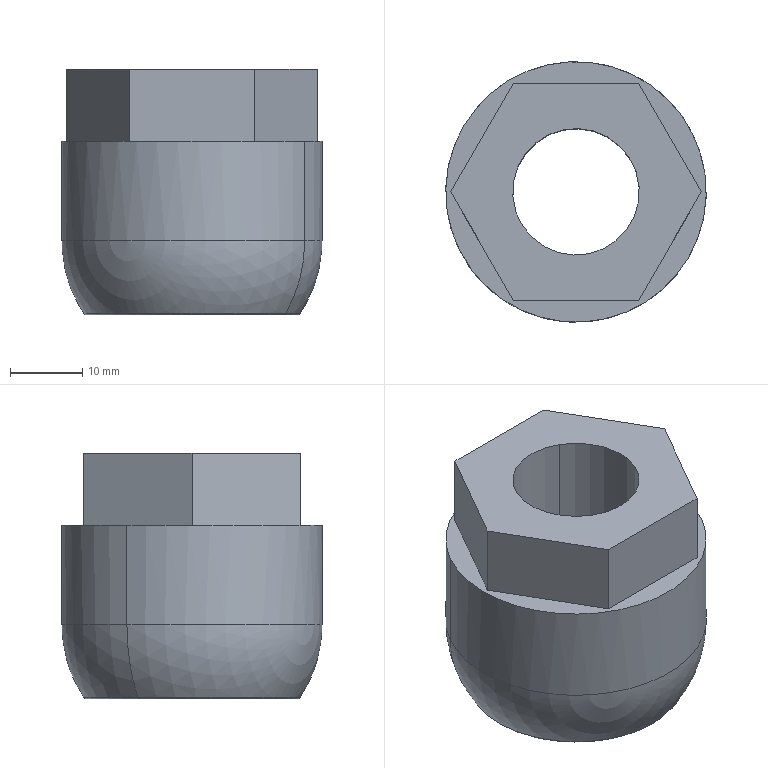Part | NX | 1 solid | 17 faces | box 36 x 36 x 34 mm | volume 22917 mm3 | plane 9 | cylinder 4 | torus 2 | sphere 2 | commonest cylinder face diameters 17.5 x2 36 x2
STEP:
#1=CARTESIAN_POINT('',(-4.375,-7.578,-34.));
#2=VERTEX_POINT('',#1);
#3=CARTESIAN_POINT('',(4.375,7.578,-34.));
#4=VERTEX_POINT('',#3);
#5=CARTESIAN_POINT('',(0.,0.,-34.));
#6=DIRECTION('',(0.,0.,1.));
#7=DIRECTION('',(0.5,0.866,0.));
#8=AXIS2_PLACEMENT_3D('',#5,#6,#7);
#9=CIRCLE('',#8,8.75);
#10=EDGE_CURVE('',#2,#4,#9,.T.);
#11=ORIENTED_EDGE('',*,*,#10,.F.);
#12=CARTESIAN_POINT('',(-4.375,-7.578,0.));
#13=VERTEX_POINT('',#12);
#14=CARTESIAN_POINT('',(-4.375,-7.578,0.));
#15=DIRECTION('',(0.,0.,1.));
#16=VECTOR('',#15,1000.);
#17=LINE('',#14,#16);
#18=EDGE_CURVE('',#13,#2,#17,.F.);
#19=ORIENTED_EDGE('',*,*,#18,.F.);
#20=CARTESIAN_POINT('',(4.375,7.578,0.));
#21=VERTEX_POINT('',#20);
#22=CARTESIAN_POINT('',(0.,0.,0.));
#23=DIRECTION('',(0.,0.,1.));
#24=DIRECTION('',(0.5,0.866,0.));
#25=AXIS2_PLACEMENT_3D('',#22,#23,#24);
#26=CIRCLE('',#25,8.75);
#27=EDGE_CURVE('',#13,#21,#26,.T.);
#28=ORIENTED_EDGE('',*,*,#27,.T.);
#29=CARTESIAN_POINT('',(4.375,7.578,0.));
#30=DIRECTION('',(0.,0.,1.));
#31=VECTOR('',#30,1000.);
#32=LINE('',#29,#31);
#33=EDGE_CURVE('',#21,#4,#32,.F.);
#34=ORIENTED_EDGE('',*,*,#33,.T.);
#35=EDGE_LOOP('',(#11,#19,#28,#34));
#36=FACE_BOUND('',#35,.T.);
#37=CARTESIAN_POINT('',(0.,0.,0.));
#38=DIRECTION('',(0.,0.,1.));
#39=DIRECTION('',(-0.5,-0.866,0.));
#40=AXIS2_PLACEMENT_3D('',#37,#38,#39);
#41=CYLINDRICAL_SURFACE('',#40,8.75);
#42=ADVANCED_FACE('',(#36),#41,.F.);
#43=CARTESIAN_POINT('',(-12.586,7.267,-34.));
#44=VERTEX_POINT('',#43);
#45=CARTESIAN_POINT('',(12.586,-7.267,-34.));
#46=VERTEX_POINT('',#45);
#47=CARTESIAN_POINT('',(0.,0.,-34.));
#48=DIRECTION('',(0.,0.,1.));
#49=DIRECTION('',(-0.866,0.5,0.));
#50=AXIS2_PLACEMENT_3D('',#47,#48,#49);
#51=CIRCLE('',#50,14.533);
#52=EDGE_CURVE('',#44,#46,#51,.T.);
#53=ORIENTED_EDGE('',*,*,#52,.T.);
#54=CARTESIAN_POINT('',(12.946,-7.474,-33.779));
#55=VERTEX_POINT('',#54);
#56=CARTESIAN_POINT('',(12.586,-7.267,-33.5));
#57=DIRECTION('',(-0.5,-0.866,0.));
#58=DIRECTION('',(-0.866,0.5,0.));
#59=AXIS2_PLACEMENT_3D('',#56,#57,#58);
#60=CIRCLE('',#59,0.5);
#61=EDGE_CURVE('',#55,#46,#60,.F.);
#62=ORIENTED_EDGE('',*,*,#61,.F.);
#63=CARTESIAN_POINT('',(-12.946,7.474,-33.779));
#64=VERTEX_POINT('',#63);
#65=CARTESIAN_POINT('',(0.,0.,-33.779));
#66=DIRECTION('',(0.,0.,1.));
#67=DIRECTION('',(-0.866,0.5,0.));
#68=AXIS2_PLACEMENT_3D('',#65,#66,#67);
#69=CIRCLE('',#68,14.948);
#70=EDGE_CURVE('',#64,#55,#69,.T.);
#71=ORIENTED_EDGE('',*,*,#70,.F.);
#72=CARTESIAN_POINT('',(-12.586,7.267,-33.5));
#73=DIRECTION('',(0.5,0.866,0.));
#74=DIRECTION('',(0.866,-0.5,0.));
#75=AXIS2_PLACEMENT_3D('',#72,#73,#74);
#76=CIRCLE('',#75,0.5);
#77=EDGE_CURVE('',#64,#44,#76,.F.);
#78=ORIENTED_EDGE('',*,*,#77,.T.);
#79=EDGE_LOOP('',(#53,#62,#71,#78));
#80=FACE_BOUND('',#79,.T.);
#81=CARTESIAN_POINT('',(0.,0.,-33.5));
#82=DIRECTION('',(0.,0.,1.));
#83=DIRECTION('',(0.866,-0.5,0.));
#84=AXIS2_PLACEMENT_3D('',#81,#82,#83);
#85=TOROIDAL_SURFACE('',#84,14.533,0.5);
#86=ADVANCED_FACE('',(#80),#85,.T.);
#87=ORIENTED_EDGE('',*,*,#70,.T.);
#88=CARTESIAN_POINT('',(15.588,-9.,-23.751));
#89=VERTEX_POINT('',#88);
#90=CARTESIAN_POINT('',(0.,0.,-23.751));
#91=DIRECTION('',(-0.5,-0.866,0.));
#92=DIRECTION('',(-0.866,0.5,0.));
#93=AXIS2_PLACEMENT_3D('',#90,#91,#92);
#94=CIRCLE('',#93,18.);
#95=EDGE_CURVE('',#89,#55,#94,.F.);
#96=ORIENTED_EDGE('',*,*,#95,.F.);
#97=CARTESIAN_POINT('',(-15.588,9.,-23.751));
#98=VERTEX_POINT('',#97);
#99=CARTESIAN_POINT('',(0.,0.,-23.751));
#100=DIRECTION('',(0.,0.,1.));
#101=DIRECTION('',(-0.866,0.5,0.));
#102=AXIS2_PLACEMENT_3D('',#99,#100,#101);
#103=CIRCLE('',#102,18.);
#104=EDGE_CURVE('',#98,#89,#103,.T.);
#105=ORIENTED_EDGE('',*,*,#104,.F.);
#106=CARTESIAN_POINT('',(0.,0.,-23.751));
#107=DIRECTION('',(0.5,0.866,0.));
#108=DIRECTION('',(0.866,-0.5,0.));
#109=AXIS2_PLACEMENT_3D('',#106,#107,#108);
#110=CIRCLE('',#109,18.);
#111=EDGE_CURVE('',#98,#64,#110,.F.);
#112=ORIENTED_EDGE('',*,*,#111,.T.);
#113=EDGE_LOOP('',(#87,#96,#105,#112));
#114=FACE_BOUND('',#113,.T.);
#115=CARTESIAN_POINT('',(0.,0.,-23.751));
#116=DIRECTION('',(-0.5,-0.866,0.));
#117=DIRECTION('',(0.866,-0.5,0.));
#118=AXIS2_PLACEMENT_3D('',#115,#116,#117);
#119=SPHERICAL_SURFACE('',#118,18.);
#120=ADVANCED_FACE('',(#114),#119,.T.);
#121=ORIENTED_EDGE('',*,*,#104,.T.);
#122=CARTESIAN_POINT('',(15.588,-9.,-10.));
#123=VERTEX_POINT('',#122);
#124=CARTESIAN_POINT('',(15.588,-9.,-35.614));
#125=DIRECTION('',(0.,0.,1.));
#126=VECTOR('',#125,1000.);
#127=LINE('',#124,#126);
#128=EDGE_CURVE('',#123,#89,#127,.F.);
#129=ORIENTED_EDGE('',*,*,#128,.F.);
#130=CARTESIAN_POINT('',(-15.588,9.,-10.));
#131=VERTEX_POINT('',#130);
#132=CARTESIAN_POINT('',(0.,0.,-10.));
#133=DIRECTION('',(0.,0.,-1.));
#134=DIRECTION('',(-0.866,0.5,0.));
#135=AXIS2_PLACEMENT_3D('',#132,#133,#134);
#136=CIRCLE('',#135,18.);
#137=EDGE_CURVE('',#123,#131,#136,.T.);
#138=ORIENTED_EDGE('',*,*,#137,.T.);
#139=CARTESIAN_POINT('',(-15.588,9.,-35.614));
#140=DIRECTION('',(0.,0.,1.));
#141=VECTOR('',#140,1000.);
#142=LINE('',#139,#141);
#143=EDGE_CURVE('',#131,#98,#142,.F.);
#144=ORIENTED_EDGE('',*,*,#143,.T.);
#145=EDGE_LOOP('',(#121,#129,#138,#144));
#146=FACE_BOUND('',#145,.T.);
#147=CARTESIAN_POINT('',(0.,0.,-35.614));
#148=DIRECTION('',(0.,0.,1.));
#149=DIRECTION('',(0.866,-0.5,0.));
#150=AXIS2_PLACEMENT_3D('',#147,#148,#149);
#151=CYLINDRICAL_SURFACE('',#150,18.);
#152=ADVANCED_FACE('',(#146),#151,.T.);
#153=ORIENTED_EDGE('',*,*,#128,.T.);
#154=CARTESIAN_POINT('',(0.,0.,-23.751));
#155=DIRECTION('',(0.,0.,1.));
#156=DIRECTION('',(-0.866,0.5,0.));
#157=AXIS2_PLACEMENT_3D('',#154,#155,#156);
#158=CIRCLE('',#157,18.);
#159=EDGE_CURVE('',#89,#98,#158,.T.);
#160=ORIENTED_EDGE('',*,*,#159,.T.);
#161=ORIENTED_EDGE('',*,*,#143,.F.);
#162=CARTESIAN_POINT('',(0.,0.,-10.));
#163=DIRECTION('',(0.,0.,-1.));
#164=DIRECTION('',(-0.866,0.5,0.));
#165=AXIS2_PLACEMENT_3D('',#162,#163,#164);
#166=CIRCLE('',#165,18.);
#167=EDGE_CURVE('',#131,#123,#166,.T.);
#168=ORIENTED_EDGE('',*,*,#167,.T.);
#169=EDGE_LOOP('',(#153,#160,#161,#168));
#170=FACE_BOUND('',#169,.T.);
#171=CARTESIAN_POINT('',(0.,0.,-35.614));
#172=DIRECTION('',(0.,0.,1.));
#173=DIRECTION('',(0.866,-0.5,0.));
#174=AXIS2_PLACEMENT_3D('',#171,#172,#173);
#175=CYLINDRICAL_SURFACE('',#174,18.);
#176=ADVANCED_FACE('',(#170),#175,.T.);
#177=CARTESIAN_POINT('',(0.,0.,0.));
#178=DIRECTION('',(0.,0.,1.));
#179=DIRECTION('',(0.5,0.866,0.));
#180=AXIS2_PLACEMENT_3D('',#177,#178,#179);
#181=CIRCLE('',#180,8.75);
#182=EDGE_CURVE('',#21,#13,#181,.T.);
#183=ORIENTED_EDGE('',*,*,#182,.F.);
#184=ORIENTED_EDGE('',*,*,#27,.F.);
#185=EDGE_LOOP('',(#183,#184));
#186=FACE_BOUND('',#185,.T.);
#187=CARTESIAN_POINT('',(-8.66,15.,0.));
#188=VERTEX_POINT('',#187);
#189=CARTESIAN_POINT('',(-17.32,0.,0.));
#190=VERTEX_POINT('',#189);
#191=CARTESIAN_POINT('',(-8.66,15.,0.));
#192=DIRECTION('',(-0.5,-0.866,0.));
#193=VECTOR('',#192,1000.);
#194=LINE('',#191,#193);
#195=EDGE_CURVE('',#188,#190,#194,.T.);
#196=ORIENTED_EDGE('',*,*,#195,.T.);
#197=CARTESIAN_POINT('',(-8.66,-15.,0.));
#198=VERTEX_POINT('',#197);
#199=CARTESIAN_POINT('',(-17.32,0.,0.));
#200=DIRECTION('',(0.5,-0.866,0.));
#201=VECTOR('',#200,1000.);
#202=LINE('',#199,#201);
#203=EDGE_CURVE('',#190,#198,#202,.T.);
#204=ORIENTED_EDGE('',*,*,#203,.T.);
#205=CARTESIAN_POINT('',(8.66,-15.,0.));
#206=VERTEX_POINT('',#205);
#207=CARTESIAN_POINT('',(-8.66,-15.,0.));
#208=DIRECTION('',(1.,0.,0.));
#209=VECTOR('',#208,1000.);
#210=LINE('',#207,#209);
#211=EDGE_CURVE('',#198,#206,#210,.T.);
#212=ORIENTED_EDGE('',*,*,#211,.T.);
#213=CARTESIAN_POINT('',(17.32,0.,0.));
#214=VERTEX_POINT('',#213);
#215=CARTESIAN_POINT('',(8.66,-15.,0.));
#216=DIRECTION('',(0.5,0.866,0.));
#217=VECTOR('',#216,1000.);
#218=LINE('',#215,#217);
#219=EDGE_CURVE('',#206,#214,#218,.T.);
#220=ORIENTED_EDGE('',*,*,#219,.T.);
#221=CARTESIAN_POINT('',(8.66,15.,0.));
#222=VERTEX_POINT('',#221);
#223=CARTESIAN_POINT('',(17.32,0.,0.));
#224=DIRECTION('',(-0.5,0.866,0.));
#225=VECTOR('',#224,1000.);
#226=LINE('',#223,#225);
#227=EDGE_CURVE('',#214,#222,#226,.T.);
#228=ORIENTED_EDGE('',*,*,#227,.T.);
#229=CARTESIAN_POINT('',(8.66,15.,0.));
#230=DIRECTION('',(-1.,0.,0.));
#231=VECTOR('',#230,1000.);
#232=LINE('',#229,#231);
#233=EDGE_CURVE('',#222,#188,#232,.T.);
#234=ORIENTED_EDGE('',*,*,#233,.T.);
#235=EDGE_LOOP('',(#196,#204,#212,#220,#228,#234));
#236=FACE_BOUND('',#235,.T.);
#237=CARTESIAN_POINT('',(0.,0.,0.));
#238=DIRECTION('',(0.,0.,1.));
#239=DIRECTION('',(0.866,-0.5,0.));
#240=AXIS2_PLACEMENT_3D('',#237,#238,#239);
#241=PLANE('',#240);
#242=ADVANCED_FACE('',(#186,#236),#241,.T.);
#243=ORIENTED_EDGE('',*,*,#95,.T.);
#244=CARTESIAN_POINT('',(0.,0.,-33.779));
#245=DIRECTION('',(0.,0.,1.));
#246=DIRECTION('',(-0.866,0.5,0.));
#247=AXIS2_PLACEMENT_3D('',#244,#245,#246);
#248=CIRCLE('',#247,14.948);
#249=EDGE_CURVE('',#55,#64,#248,.T.);
#250=ORIENTED_EDGE('',*,*,#249,.T.);
#251=ORIENTED_EDGE('',*,*,#111,.F.);
#252=ORIENTED_EDGE('',*,*,#159,.F.);
#253=EDGE_LOOP('',(#243,#250,#251,#252));
#254=FACE_BOUND('',#253,.T.);
#255=CARTESIAN_POINT('',(0.,0.,-23.751));
#256=DIRECTION('',(-0.5,-0.866,0.));
#257=DIRECTION('',(0.866,-0.5,0.));
#258=AXIS2_PLACEMENT_3D('',#255,#256,#257);
#259=SPHERICAL_SURFACE('',#258,18.);
#260=ADVANCED_FACE('',(#254),#259,.T.);
#261=ORIENTED_EDGE('',*,*,#61,.T.);
#262=CARTESIAN_POINT('',(0.,0.,-34.));
#263=DIRECTION('',(0.,0.,1.));
#264=DIRECTION('',(-0.866,0.5,0.));
#265=AXIS2_PLACEMENT_3D('',#262,#263,#264);
#266=CIRCLE('',#265,14.533);
#267=EDGE_CURVE('',#46,#44,#266,.T.);
#268=ORIENTED_EDGE('',*,*,#267,.T.);
#269=ORIENTED_EDGE('',*,*,#77,.F.);
#270=ORIENTED_EDGE('',*,*,#249,.F.);
#271=EDGE_LOOP('',(#261,#268,#269,#270));
#272=FACE_BOUND('',#271,.T.);
#273=CARTESIAN_POINT('',(0.,0.,-33.5));
#274=DIRECTION('',(0.,0.,1.));
#275=DIRECTION('',(0.866,-0.5,0.));
#276=AXIS2_PLACEMENT_3D('',#273,#274,#275);
#277=TOROIDAL_SURFACE('',#276,14.533,0.5);
#278=ADVANCED_FACE('',(#272),#277,.T.);
#279=CARTESIAN_POINT('',(0.,0.,-34.));
#280=DIRECTION('',(0.,0.,1.));
#281=DIRECTION('',(0.5,0.866,0.));
#282=AXIS2_PLACEMENT_3D('',#279,#280,#281);
#283=CIRCLE('',#282,8.75);
#284=EDGE_CURVE('',#4,#2,#283,.T.);
#285=ORIENTED_EDGE('',*,*,#284,.T.);
#286=ORIENTED_EDGE('',*,*,#10,.T.);
#287=EDGE_LOOP('',(#285,#286));
#288=FACE_BOUND('',#287,.T.);
#289=ORIENTED_EDGE('',*,*,#52,.F.);
#290=ORIENTED_EDGE('',*,*,#267,.F.);
#291=EDGE_LOOP('',(#289,#290));
#292=FACE_BOUND('',#291,.T.);
#293=CARTESIAN_POINT('',(-12.586,7.267,-34.));
#294=DIRECTION('',(0.,0.,-1.));
#295=DIRECTION('',(-0.866,0.5,0.));
#296=AXIS2_PLACEMENT_3D('',#293,#294,#295);
#297=PLANE('',#296);
#298=ADVANCED_FACE('',(#288,#292),#297,.T.);
#299=ORIENTED_EDGE('',*,*,#18,.T.);
#300=ORIENTED_EDGE('',*,*,#284,.F.);
#301=ORIENTED_EDGE('',*,*,#33,.F.);
#302=ORIENTED_EDGE('',*,*,#182,.T.);
#303=EDGE_LOOP('',(#299,#300,#301,#302));
#304=FACE_BOUND('',#303,.T.);
#305=CARTESIAN_POINT('',(0.,0.,0.));
#306=DIRECTION('',(0.,0.,1.));
#307=DIRECTION('',(-0.5,-0.866,0.));
#308=AXIS2_PLACEMENT_3D('',#305,#306,#307);
#309=CYLINDRICAL_SURFACE('',#308,8.75);
#310=ADVANCED_FACE('',(#304),#309,.F.);
#311=ORIENTED_EDGE('',*,*,#167,.F.);
#312=ORIENTED_EDGE('',*,*,#137,.F.);
#313=EDGE_LOOP('',(#311,#312));
#314=FACE_BOUND('',#313,.T.);
#315=CARTESIAN_POINT('',(-8.66,15.,-10.));
#316=VERTEX_POINT('',#315);
#317=CARTESIAN_POINT('',(-17.32,0.,-10.));
#318=VERTEX_POINT('',#317);
#319=CARTESIAN_POINT('',(-8.66,15.,-10.));
#320=DIRECTION('',(-0.5,-0.866,0.));
#321=VECTOR('',#320,1000.);
#322=LINE('',#319,#321);
#323=EDGE_CURVE('',#316,#318,#322,.T.);
#324=ORIENTED_EDGE('',*,*,#323,.F.);
#325=CARTESIAN_POINT('',(8.66,15.,-10.));
#326=VERTEX_POINT('',#325);
#327=CARTESIAN_POINT('',(8.66,15.,-10.));
#328=DIRECTION('',(-1.,0.,0.));
#329=VECTOR('',#328,1000.);
#330=LINE('',#327,#329);
#331=EDGE_CURVE('',#326,#316,#330,.T.);
#332=ORIENTED_EDGE('',*,*,#331,.F.);
#333=CARTESIAN_POINT('',(17.32,0.,-10.));
#334=VERTEX_POINT('',#333);
#335=CARTESIAN_POINT('',(17.32,0.,-10.));
#336=DIRECTION('',(-0.5,0.866,0.));
#337=VECTOR('',#336,1000.);
#338=LINE('',#335,#337);
#339=EDGE_CURVE('',#334,#326,#338,.T.);
#340=ORIENTED_EDGE('',*,*,#339,.F.);
#341=CARTESIAN_POINT('',(8.66,-15.,-10.));
#342=VERTEX_POINT('',#341);
#343=CARTESIAN_POINT('',(8.66,-15.,-10.));
#344=DIRECTION('',(0.5,0.866,0.));
#345=VECTOR('',#344,1000.);
#346=LINE('',#343,#345);
#347=EDGE_CURVE('',#342,#334,#346,.T.);
#348=ORIENTED_EDGE('',*,*,#347,.F.);
#349=CARTESIAN_POINT('',(-8.66,-15.,-10.));
#350=VERTEX_POINT('',#349);
#351=CARTESIAN_POINT('',(-8.66,-15.,-10.));
#352=DIRECTION('',(1.,0.,0.));
#353=VECTOR('',#352,1000.);
#354=LINE('',#351,#353);
#355=EDGE_CURVE('',#350,#342,#354,.T.);
#356=ORIENTED_EDGE('',*,*,#355,.F.);
#357=CARTESIAN_POINT('',(-17.32,0.,-10.));
#358=DIRECTION('',(0.5,-0.866,0.));
#359=VECTOR('',#358,1000.);
#360=LINE('',#357,#359);
#361=EDGE_CURVE('',#318,#350,#360,.T.);
#362=ORIENTED_EDGE('',*,*,#361,.F.);
#363=EDGE_LOOP('',(#324,#332,#340,#348,#356,#362));
#364=FACE_BOUND('',#363,.T.);
#365=CARTESIAN_POINT('',(0.,0.,-10.));
#366=DIRECTION('',(0.,0.,1.));
#367=DIRECTION('',(0.866,-0.5,0.));
#368=AXIS2_PLACEMENT_3D('',#365,#366,#367);
#369=PLANE('',#368);
#370=ADVANCED_FACE('',(#314,#364),#369,.T.);
#371=ORIENTED_EDGE('',*,*,#203,.F.);
#372=CARTESIAN_POINT('',(-17.32,0.,-10.));
#373=DIRECTION('',(0.,0.,1.));
#374=VECTOR('',#373,1000.);
#375=LINE('',#372,#374);
#376=EDGE_CURVE('',#318,#190,#375,.T.);
#377=ORIENTED_EDGE('',*,*,#376,.F.);
#378=ORIENTED_EDGE('',*,*,#361,.T.);
#379=CARTESIAN_POINT('',(-8.66,-15.,-10.));
#380=DIRECTION('',(0.,0.,1.));
#381=VECTOR('',#380,1000.);
#382=LINE('',#379,#381);
#383=EDGE_CURVE('',#350,#198,#382,.T.);
#384=ORIENTED_EDGE('',*,*,#383,.T.);
#385=EDGE_LOOP('',(#371,#377,#378,#384));
#386=FACE_BOUND('',#385,.T.);
#387=CARTESIAN_POINT('',(-17.32,0.,-10.));
#388=DIRECTION('',(-0.866,-0.5,0.));
#389=DIRECTION('',(0.5,-0.866,0.));
#390=AXIS2_PLACEMENT_3D('',#387,#388,#389);
#391=PLANE('',#390);
#392=ADVANCED_FACE('',(#386),#391,.T.);
#393=ORIENTED_EDGE('',*,*,#195,.F.);
#394=CARTESIAN_POINT('',(-8.66,15.,-10.));
#395=DIRECTION('',(0.,0.,1.));
#396=VECTOR('',#395,1000.);
#397=LINE('',#394,#396);
#398=EDGE_CURVE('',#316,#188,#397,.T.);
#399=ORIENTED_EDGE('',*,*,#398,.F.);
#400=ORIENTED_EDGE('',*,*,#323,.T.);
#401=ORIENTED_EDGE('',*,*,#376,.T.);
#402=EDGE_LOOP('',(#393,#399,#400,#401));
#403=FACE_BOUND('',#402,.T.);
#404=CARTESIAN_POINT('',(-8.66,15.,-10.));
#405=DIRECTION('',(-0.866,0.5,0.));
#406=DIRECTION('',(-0.5,-0.866,0.));
#407=AXIS2_PLACEMENT_3D('',#404,#405,#406);
#408=PLANE('',#407);
#409=ADVANCED_FACE('',(#403),#408,.T.);
#410=ORIENTED_EDGE('',*,*,#233,.F.);
#411=CARTESIAN_POINT('',(8.66,15.,-10.));
#412=DIRECTION('',(0.,0.,1.));
#413=VECTOR('',#412,1000.);
#414=LINE('',#411,#413);
#415=EDGE_CURVE('',#326,#222,#414,.T.);
#416=ORIENTED_EDGE('',*,*,#415,.F.);
#417=ORIENTED_EDGE('',*,*,#331,.T.);
#418=ORIENTED_EDGE('',*,*,#398,.T.);
#419=EDGE_LOOP('',(#410,#416,#417,#418));
#420=FACE_BOUND('',#419,.T.);
#421=CARTESIAN_POINT('',(8.66,15.,-10.));
#422=DIRECTION('',(0.,1.,0.));
#423=DIRECTION('',(-1.,0.,0.));
#424=AXIS2_PLACEMENT_3D('',#421,#422,#423);
#425=PLANE('',#424);
#426=ADVANCED_FACE('',(#420),#425,.T.);
#427=ORIENTED_EDGE('',*,*,#227,.F.);
#428=CARTESIAN_POINT('',(17.32,0.,-10.));
#429=DIRECTION('',(0.,0.,1.));
#430=VECTOR('',#429,1000.);
#431=LINE('',#428,#430);
#432=EDGE_CURVE('',#334,#214,#431,.T.);
#433=ORIENTED_EDGE('',*,*,#432,.F.);
#434=ORIENTED_EDGE('',*,*,#339,.T.);
#435=ORIENTED_EDGE('',*,*,#415,.T.);
#436=EDGE_LOOP('',(#427,#433,#434,#435));
#437=FACE_BOUND('',#436,.T.);
#438=CARTESIAN_POINT('',(17.32,0.,-10.));
#439=DIRECTION('',(0.866,0.5,0.));
#440=DIRECTION('',(-0.5,0.866,0.));
#441=AXIS2_PLACEMENT_3D('',#438,#439,#440);
#442=PLANE('',#441);
#443=ADVANCED_FACE('',(#437),#442,.T.);
#444=ORIENTED_EDGE('',*,*,#219,.F.);
#445=CARTESIAN_POINT('',(8.66,-15.,-10.));
#446=DIRECTION('',(0.,0.,1.));
#447=VECTOR('',#446,1000.);
#448=LINE('',#445,#447);
#449=EDGE_CURVE('',#342,#206,#448,.T.);
#450=ORIENTED_EDGE('',*,*,#449,.F.);
#451=ORIENTED_EDGE('',*,*,#347,.T.);
#452=ORIENTED_EDGE('',*,*,#432,.T.);
#453=EDGE_LOOP('',(#444,#450,#451,#452));
#454=FACE_BOUND('',#453,.T.);
#455=CARTESIAN_POINT('',(8.66,-15.,-10.));
#456=DIRECTION('',(0.866,-0.5,0.));
#457=DIRECTION('',(0.,0.,-1.));
#458=AXIS2_PLACEMENT_3D('',#455,#456,#457);
#459=PLANE('',#458);
#460=ADVANCED_FACE('',(#454),#459,.T.);
#461=ORIENTED_EDGE('',*,*,#211,.F.);
#462=ORIENTED_EDGE('',*,*,#383,.F.);
#463=ORIENTED_EDGE('',*,*,#355,.T.);
#464=ORIENTED_EDGE('',*,*,#449,.T.);
#465=EDGE_LOOP('',(#461,#462,#463,#464));
#466=FACE_BOUND('',#465,.T.);
#467=CARTESIAN_POINT('',(-8.66,-15.,-10.));
#468=DIRECTION('',(0.,-1.,0.));
#469=DIRECTION('',(1.,0.,0.));
#470=AXIS2_PLACEMENT_3D('',#467,#468,#469);
#471=PLANE('',#470);
#472=ADVANCED_FACE('',(#466),#471,.T.);
#473=CLOSED_SHELL('',(#42,#86,#120,#152,#176,#242,#260,#278,#298,#310,#370,#392,#409,#426,#443,#460,#472));
#474=MANIFOLD_SOLID_BREP('',#473);
#475=(LENGTH_UNIT()NAMED_UNIT(*)SI_UNIT(.MILLI.,.METRE.));
#476=UNCERTAINTY_MEASURE_WITH_UNIT(LENGTH_MEASURE(0.00001),#475,'','');
#477=(NAMED_UNIT(*)PLANE_ANGLE_UNIT()SI_UNIT($,.RADIAN.));
#478=(NAMED_UNIT(*)SI_UNIT($,.STERADIAN.)SOLID_ANGLE_UNIT());
#479=(GEOMETRIC_REPRESENTATION_CONTEXT(3)GLOBAL_UNCERTAINTY_ASSIGNED_CONTEXT((#476))GLOBAL_UNIT_ASSIGNED_CONTEXT((#475,#477,#478))REPRESENTATION_CONTEXT('',''));
#480=ADVANCED_BREP_SHAPE_REPRESENTATION('',(#474),#479);